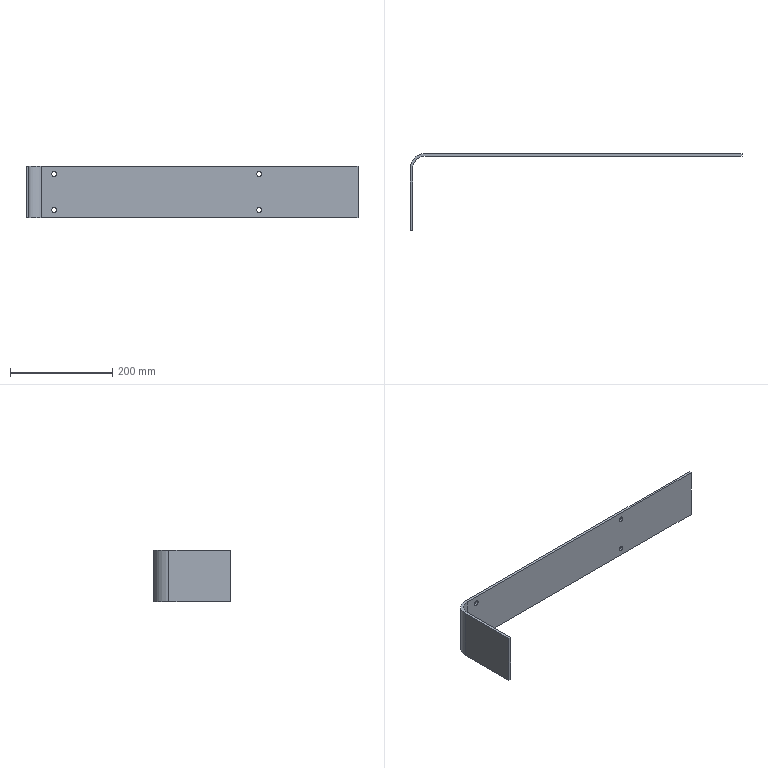Part | SolidWorks | features ExtruThin 1, ICE 1, LPattern 1 | 1 solid | 18 faces | box 648 x 150 x 100 mm | volume 389028 mm3 | cylinder 10 | plane 8 | commonest cylinder face diameters 10 x8 50 x1 60 x1
STEP:
#1=CARTESIAN_POINT('',(455.,150.,10.));
#2=VERTEX_POINT('',#1);
#3=CARTESIAN_POINT('',(455.,150.,20.));
#4=VERTEX_POINT('',#3);
#5=CARTESIAN_POINT('',(455.,150.,15.));
#6=DIRECTION('',(0.,1.,0.));
#7=DIRECTION('',(0.,0.,1.));
#8=AXIS2_PLACEMENT_3D('',#5,#6,#7);
#9=CIRCLE('',#8,5.);
#10=EDGE_CURVE('',#2,#4,#9,.T.);
#11=ORIENTED_EDGE('',*,*,#10,.T.);
#12=CARTESIAN_POINT('',(455.,145.,20.));
#13=VERTEX_POINT('',#12);
#14=CARTESIAN_POINT('',(455.,155.,20.));
#15=DIRECTION('',(0.,-1.,0.));
#16=VECTOR('',#15,1000.);
#17=LINE('',#14,#16);
#18=EDGE_CURVE('',#4,#13,#17,.T.);
#19=ORIENTED_EDGE('',*,*,#18,.T.);
#20=CARTESIAN_POINT('',(455.,145.,10.));
#21=VERTEX_POINT('',#20);
#22=CARTESIAN_POINT('',(455.,145.,15.));
#23=DIRECTION('',(0.,-1.,0.));
#24=DIRECTION('',(0.,0.,-1.));
#25=AXIS2_PLACEMENT_3D('',#22,#23,#24);
#26=CIRCLE('',#25,5.);
#27=EDGE_CURVE('',#13,#21,#26,.T.);
#28=ORIENTED_EDGE('',*,*,#27,.T.);
#29=CARTESIAN_POINT('',(455.,155.,10.));
#30=DIRECTION('',(0.,-1.,0.));
#31=VECTOR('',#30,1000.);
#32=LINE('',#29,#31);
#33=EDGE_CURVE('',#2,#21,#32,.T.);
#34=ORIENTED_EDGE('',*,*,#33,.F.);
#35=EDGE_LOOP('',(#11,#19,#28,#34));
#36=FACE_OUTER_BOUND('',#35,.T.);
#37=CARTESIAN_POINT('',(455.,155.,15.));
#38=DIRECTION('',(0.,-1.,0.));
#39=DIRECTION('',(0.,0.,-1.));
#40=AXIS2_PLACEMENT_3D('',#37,#38,#39);
#41=CYLINDRICAL_SURFACE('',#40,5.);
#42=ADVANCED_FACE('',(#36),#41,.F.);
#43=CARTESIAN_POINT('',(55.,150.,10.));
#44=VERTEX_POINT('',#43);
#45=CARTESIAN_POINT('',(55.,150.,20.));
#46=VERTEX_POINT('',#45);
#47=CARTESIAN_POINT('',(55.,150.,15.));
#48=DIRECTION('',(0.,1.,0.));
#49=DIRECTION('',(0.,0.,1.));
#50=AXIS2_PLACEMENT_3D('',#47,#48,#49);
#51=CIRCLE('',#50,5.);
#52=EDGE_CURVE('',#44,#46,#51,.T.);
#53=ORIENTED_EDGE('',*,*,#52,.T.);
#54=CARTESIAN_POINT('',(55.,145.,20.));
#55=VERTEX_POINT('',#54);
#56=CARTESIAN_POINT('',(55.,155.,20.));
#57=DIRECTION('',(0.,-1.,0.));
#58=VECTOR('',#57,1000.);
#59=LINE('',#56,#58);
#60=EDGE_CURVE('',#46,#55,#59,.T.);
#61=ORIENTED_EDGE('',*,*,#60,.T.);
#62=CARTESIAN_POINT('',(55.,145.,10.));
#63=VERTEX_POINT('',#62);
#64=CARTESIAN_POINT('',(55.,145.,15.));
#65=DIRECTION('',(0.,-1.,0.));
#66=DIRECTION('',(0.,0.,-1.));
#67=AXIS2_PLACEMENT_3D('',#64,#65,#66);
#68=CIRCLE('',#67,5.);
#69=EDGE_CURVE('',#55,#63,#68,.T.);
#70=ORIENTED_EDGE('',*,*,#69,.T.);
#71=CARTESIAN_POINT('',(55.,155.,10.));
#72=DIRECTION('',(0.,-1.,0.));
#73=VECTOR('',#72,1000.);
#74=LINE('',#71,#73);
#75=EDGE_CURVE('',#44,#63,#74,.T.);
#76=ORIENTED_EDGE('',*,*,#75,.F.);
#77=EDGE_LOOP('',(#53,#61,#70,#76));
#78=FACE_OUTER_BOUND('',#77,.T.);
#79=CARTESIAN_POINT('',(55.,155.,15.));
#80=DIRECTION('',(0.,-1.,0.));
#81=DIRECTION('',(0.,0.,-1.));
#82=AXIS2_PLACEMENT_3D('',#79,#80,#81);
#83=CYLINDRICAL_SURFACE('',#82,5.);
#84=ADVANCED_FACE('',(#78),#83,.F.);
#85=CARTESIAN_POINT('',(455.,150.,80.));
#86=VERTEX_POINT('',#85);
#87=CARTESIAN_POINT('',(455.,150.,90.));
#88=VERTEX_POINT('',#87);
#89=CARTESIAN_POINT('',(455.,150.,85.));
#90=DIRECTION('',(0.,1.,0.));
#91=DIRECTION('',(0.,0.,1.));
#92=AXIS2_PLACEMENT_3D('',#89,#90,#91);
#93=CIRCLE('',#92,5.);
#94=EDGE_CURVE('',#86,#88,#93,.T.);
#95=ORIENTED_EDGE('',*,*,#94,.T.);
#96=CARTESIAN_POINT('',(455.,145.,90.));
#97=VERTEX_POINT('',#96);
#98=CARTESIAN_POINT('',(455.,155.,90.));
#99=DIRECTION('',(0.,-1.,0.));
#100=VECTOR('',#99,1000.);
#101=LINE('',#98,#100);
#102=EDGE_CURVE('',#88,#97,#101,.T.);
#103=ORIENTED_EDGE('',*,*,#102,.T.);
#104=CARTESIAN_POINT('',(455.,145.,80.));
#105=VERTEX_POINT('',#104);
#106=CARTESIAN_POINT('',(455.,145.,85.));
#107=DIRECTION('',(0.,-1.,0.));
#108=DIRECTION('',(0.,0.,-1.));
#109=AXIS2_PLACEMENT_3D('',#106,#107,#108);
#110=CIRCLE('',#109,5.);
#111=EDGE_CURVE('',#97,#105,#110,.T.);
#112=ORIENTED_EDGE('',*,*,#111,.T.);
#113=CARTESIAN_POINT('',(455.,155.,80.));
#114=DIRECTION('',(0.,-1.,0.));
#115=VECTOR('',#114,1000.);
#116=LINE('',#113,#115);
#117=EDGE_CURVE('',#86,#105,#116,.T.);
#118=ORIENTED_EDGE('',*,*,#117,.F.);
#119=EDGE_LOOP('',(#95,#103,#112,#118));
#120=FACE_OUTER_BOUND('',#119,.T.);
#121=CARTESIAN_POINT('',(455.,155.,85.));
#122=DIRECTION('',(0.,-1.,0.));
#123=DIRECTION('',(0.,0.,-1.));
#124=AXIS2_PLACEMENT_3D('',#121,#122,#123);
#125=CYLINDRICAL_SURFACE('',#124,5.);
#126=ADVANCED_FACE('',(#120),#125,.F.);
#127=CARTESIAN_POINT('',(55.,150.,80.));
#128=VERTEX_POINT('',#127);
#129=CARTESIAN_POINT('',(55.,150.,90.));
#130=VERTEX_POINT('',#129);
#131=CARTESIAN_POINT('',(55.,150.,85.));
#132=DIRECTION('',(0.,1.,0.));
#133=DIRECTION('',(0.,0.,1.));
#134=AXIS2_PLACEMENT_3D('',#131,#132,#133);
#135=CIRCLE('',#134,5.);
#136=EDGE_CURVE('',#128,#130,#135,.T.);
#137=ORIENTED_EDGE('',*,*,#136,.T.);
#138=CARTESIAN_POINT('',(55.,145.,90.));
#139=VERTEX_POINT('',#138);
#140=CARTESIAN_POINT('',(55.,155.,90.));
#141=DIRECTION('',(0.,-1.,0.));
#142=VECTOR('',#141,1000.);
#143=LINE('',#140,#142);
#144=EDGE_CURVE('',#130,#139,#143,.T.);
#145=ORIENTED_EDGE('',*,*,#144,.T.);
#146=CARTESIAN_POINT('',(55.,145.,80.));
#147=VERTEX_POINT('',#146);
#148=CARTESIAN_POINT('',(55.,145.,85.));
#149=DIRECTION('',(0.,-1.,0.));
#150=DIRECTION('',(0.,0.,-1.));
#151=AXIS2_PLACEMENT_3D('',#148,#149,#150);
#152=CIRCLE('',#151,5.);
#153=EDGE_CURVE('',#139,#147,#152,.T.);
#154=ORIENTED_EDGE('',*,*,#153,.T.);
#155=CARTESIAN_POINT('',(55.,155.,80.));
#156=DIRECTION('',(0.,-1.,0.));
#157=VECTOR('',#156,1000.);
#158=LINE('',#155,#157);
#159=EDGE_CURVE('',#128,#147,#158,.T.);
#160=ORIENTED_EDGE('',*,*,#159,.F.);
#161=EDGE_LOOP('',(#137,#145,#154,#160));
#162=FACE_OUTER_BOUND('',#161,.T.);
#163=CARTESIAN_POINT('',(55.,155.,85.));
#164=DIRECTION('',(0.,-1.,0.));
#165=DIRECTION('',(0.,0.,-1.));
#166=AXIS2_PLACEMENT_3D('',#163,#164,#165);
#167=CYLINDRICAL_SURFACE('',#166,5.);
#168=ADVANCED_FACE('',(#162),#167,.F.);
#169=CARTESIAN_POINT('',(455.,145.,85.));
#170=DIRECTION('',(0.,-1.,0.));
#171=DIRECTION('',(0.,0.,-1.));
#172=AXIS2_PLACEMENT_3D('',#169,#170,#171);
#173=CIRCLE('',#172,5.);
#174=EDGE_CURVE('',#105,#97,#173,.T.);
#175=ORIENTED_EDGE('',*,*,#174,.F.);
#176=ORIENTED_EDGE('',*,*,#111,.F.);
#177=EDGE_LOOP('',(#175,#176));
#178=FACE_BOUND('',#177,.T.);
#179=CARTESIAN_POINT('',(55.,145.,85.));
#180=DIRECTION('',(0.,-1.,0.));
#181=DIRECTION('',(0.,0.,-1.));
#182=AXIS2_PLACEMENT_3D('',#179,#180,#181);
#183=CIRCLE('',#182,5.);
#184=EDGE_CURVE('',#147,#139,#183,.T.);
#185=ORIENTED_EDGE('',*,*,#184,.F.);
#186=ORIENTED_EDGE('',*,*,#153,.F.);
#187=EDGE_LOOP('',(#185,#186));
#188=FACE_BOUND('',#187,.T.);
#189=CARTESIAN_POINT('',(30.,145.,0.));
#190=VERTEX_POINT('',#189);
#191=CARTESIAN_POINT('',(648.,145.,0.));
#192=VERTEX_POINT('',#191);
#193=CARTESIAN_POINT('',(30.,145.,0.));
#194=DIRECTION('',(1.,0.,0.));
#195=VECTOR('',#194,1000.);
#196=LINE('',#193,#195);
#197=EDGE_CURVE('',#190,#192,#196,.T.);
#198=ORIENTED_EDGE('',*,*,#197,.T.);
#199=CARTESIAN_POINT('',(648.,145.,100.));
#200=VERTEX_POINT('',#199);
#201=CARTESIAN_POINT('',(648.,145.,100.));
#202=DIRECTION('',(0.,0.,-1.));
#203=VECTOR('',#202,1000.);
#204=LINE('',#201,#203);
#205=EDGE_CURVE('',#200,#192,#204,.T.);
#206=ORIENTED_EDGE('',*,*,#205,.F.);
#207=CARTESIAN_POINT('',(30.,145.,100.));
#208=VERTEX_POINT('',#207);
#209=CARTESIAN_POINT('',(30.,145.,100.));
#210=DIRECTION('',(1.,0.,0.));
#211=VECTOR('',#210,1000.);
#212=LINE('',#209,#211);
#213=EDGE_CURVE('',#208,#200,#212,.T.);
#214=ORIENTED_EDGE('',*,*,#213,.F.);
#215=CARTESIAN_POINT('',(30.,145.,100.));
#216=DIRECTION('',(0.,0.,-1.));
#217=VECTOR('',#216,1000.);
#218=LINE('',#215,#217);
#219=EDGE_CURVE('',#208,#190,#218,.T.);
#220=ORIENTED_EDGE('',*,*,#219,.T.);
#221=EDGE_LOOP('',(#198,#206,#214,#220));
#222=FACE_OUTER_BOUND('',#221,.T.);
#223=CARTESIAN_POINT('',(55.,145.,15.));
#224=DIRECTION('',(0.,-1.,0.));
#225=DIRECTION('',(0.,0.,-1.));
#226=AXIS2_PLACEMENT_3D('',#223,#224,#225);
#227=CIRCLE('',#226,5.);
#228=EDGE_CURVE('',#63,#55,#227,.T.);
#229=ORIENTED_EDGE('',*,*,#228,.F.);
#230=ORIENTED_EDGE('',*,*,#69,.F.);
#231=EDGE_LOOP('',(#229,#230));
#232=FACE_BOUND('',#231,.T.);
#233=CARTESIAN_POINT('',(455.,145.,15.));
#234=DIRECTION('',(0.,-1.,0.));
#235=DIRECTION('',(0.,0.,-1.));
#236=AXIS2_PLACEMENT_3D('',#233,#234,#235);
#237=CIRCLE('',#236,5.);
#238=EDGE_CURVE('',#21,#13,#237,.T.);
#239=ORIENTED_EDGE('',*,*,#238,.F.);
#240=ORIENTED_EDGE('',*,*,#27,.F.);
#241=EDGE_LOOP('',(#239,#240));
#242=FACE_BOUND('',#241,.T.);
#243=CARTESIAN_POINT('',(30.,145.,100.));
#244=DIRECTION('',(0.,1.,0.));
#245=DIRECTION('',(0.,0.,1.));
#246=AXIS2_PLACEMENT_3D('',#243,#244,#245);
#247=PLANE('',#246);
#248=ADVANCED_FACE('',(#178,#188,#222,#232,#242),#247,.F.);
#249=CARTESIAN_POINT('',(648.,150.,0.));
#250=VERTEX_POINT('',#249);
#251=CARTESIAN_POINT('',(648.,150.,0.));
#252=DIRECTION('',(0.,-1.,0.));
#253=VECTOR('',#252,1000.);
#254=LINE('',#251,#253);
#255=EDGE_CURVE('',#250,#192,#254,.T.);
#256=ORIENTED_EDGE('',*,*,#255,.F.);
#257=CARTESIAN_POINT('',(648.,150.,100.));
#258=VERTEX_POINT('',#257);
#259=CARTESIAN_POINT('',(648.,150.,100.));
#260=DIRECTION('',(0.,0.,-1.));
#261=VECTOR('',#260,1000.);
#262=LINE('',#259,#261);
#263=EDGE_CURVE('',#258,#250,#262,.T.);
#264=ORIENTED_EDGE('',*,*,#263,.F.);
#265=CARTESIAN_POINT('',(648.,150.,100.));
#266=DIRECTION('',(0.,-1.,0.));
#267=VECTOR('',#266,1000.);
#268=LINE('',#265,#267);
#269=EDGE_CURVE('',#258,#200,#268,.T.);
#270=ORIENTED_EDGE('',*,*,#269,.T.);
#271=ORIENTED_EDGE('',*,*,#205,.T.);
#272=EDGE_LOOP('',(#256,#264,#270,#271));
#273=FACE_OUTER_BOUND('',#272,.T.);
#274=CARTESIAN_POINT('',(648.,150.,100.));
#275=DIRECTION('',(1.,0.,0.));
#276=DIRECTION('',(0.,0.,-1.));
#277=AXIS2_PLACEMENT_3D('',#274,#275,#276);
#278=PLANE('',#277);
#279=ADVANCED_FACE('',(#273),#278,.T.);
#280=ORIENTED_EDGE('',*,*,#94,.F.);
#281=CARTESIAN_POINT('',(455.,150.,85.));
#282=DIRECTION('',(0.,1.,0.));
#283=DIRECTION('',(0.,0.,1.));
#284=AXIS2_PLACEMENT_3D('',#281,#282,#283);
#285=CIRCLE('',#284,5.);
#286=EDGE_CURVE('',#88,#86,#285,.T.);
#287=ORIENTED_EDGE('',*,*,#286,.F.);
#288=EDGE_LOOP('',(#280,#287));
#289=FACE_BOUND('',#288,.T.);
#290=ORIENTED_EDGE('',*,*,#136,.F.);
#291=CARTESIAN_POINT('',(55.,150.,85.));
#292=DIRECTION('',(0.,1.,0.));
#293=DIRECTION('',(0.,0.,1.));
#294=AXIS2_PLACEMENT_3D('',#291,#292,#293);
#295=CIRCLE('',#294,5.);
#296=EDGE_CURVE('',#130,#128,#295,.T.);
#297=ORIENTED_EDGE('',*,*,#296,.F.);
#298=EDGE_LOOP('',(#290,#297));
#299=FACE_BOUND('',#298,.T.);
#300=CARTESIAN_POINT('',(30.,150.,0.));
#301=VERTEX_POINT('',#300);
#302=CARTESIAN_POINT('',(30.,150.,0.));
#303=DIRECTION('',(1.,0.,0.));
#304=VECTOR('',#303,1000.);
#305=LINE('',#302,#304);
#306=EDGE_CURVE('',#301,#250,#305,.T.);
#307=ORIENTED_EDGE('',*,*,#306,.F.);
#308=CARTESIAN_POINT('',(30.,150.,100.));
#309=VERTEX_POINT('',#308);
#310=CARTESIAN_POINT('',(30.,150.,100.));
#311=DIRECTION('',(0.,0.,-1.));
#312=VECTOR('',#311,1000.);
#313=LINE('',#310,#312);
#314=EDGE_CURVE('',#309,#301,#313,.T.);
#315=ORIENTED_EDGE('',*,*,#314,.F.);
#316=CARTESIAN_POINT('',(30.,150.,100.));
#317=DIRECTION('',(1.,0.,0.));
#318=VECTOR('',#317,1000.);
#319=LINE('',#316,#318);
#320=EDGE_CURVE('',#309,#258,#319,.T.);
#321=ORIENTED_EDGE('',*,*,#320,.T.);
#322=ORIENTED_EDGE('',*,*,#263,.T.);
#323=EDGE_LOOP('',(#307,#315,#321,#322));
#324=FACE_OUTER_BOUND('',#323,.T.);
#325=ORIENTED_EDGE('',*,*,#52,.F.);
#326=CARTESIAN_POINT('',(55.,150.,15.));
#327=DIRECTION('',(0.,1.,0.));
#328=DIRECTION('',(0.,0.,1.));
#329=AXIS2_PLACEMENT_3D('',#326,#327,#328);
#330=CIRCLE('',#329,5.);
#331=EDGE_CURVE('',#46,#44,#330,.T.);
#332=ORIENTED_EDGE('',*,*,#331,.F.);
#333=EDGE_LOOP('',(#325,#332));
#334=FACE_BOUND('',#333,.T.);
#335=ORIENTED_EDGE('',*,*,#10,.F.);
#336=CARTESIAN_POINT('',(455.,150.,15.));
#337=DIRECTION('',(0.,1.,0.));
#338=DIRECTION('',(0.,0.,1.));
#339=AXIS2_PLACEMENT_3D('',#336,#337,#338);
#340=CIRCLE('',#339,5.);
#341=EDGE_CURVE('',#4,#2,#340,.T.);
#342=ORIENTED_EDGE('',*,*,#341,.F.);
#343=EDGE_LOOP('',(#335,#342));
#344=FACE_BOUND('',#343,.T.);
#345=CARTESIAN_POINT('',(30.,150.,100.));
#346=DIRECTION('',(0.,1.,0.));
#347=DIRECTION('',(0.,0.,1.));
#348=AXIS2_PLACEMENT_3D('',#345,#346,#347);
#349=PLANE('',#348);
#350=ADVANCED_FACE('',(#289,#299,#324,#334,#344),#349,.T.);
#351=CARTESIAN_POINT('',(0.,120.,0.));
#352=VERTEX_POINT('',#351);
#353=CARTESIAN_POINT('',(30.,120.,0.));
#354=DIRECTION('',(0.,0.,-1.));
#355=DIRECTION('',(1.,0.,0.));
#356=AXIS2_PLACEMENT_3D('',#353,#354,#355);
#357=CIRCLE('',#356,30.);
#358=EDGE_CURVE('',#352,#301,#357,.T.);
#359=ORIENTED_EDGE('',*,*,#358,.F.);
#360=CARTESIAN_POINT('',(0.,120.,100.));
#361=VERTEX_POINT('',#360);
#362=CARTESIAN_POINT('',(0.,120.,100.));
#363=DIRECTION('',(0.,0.,-1.));
#364=VECTOR('',#363,1000.);
#365=LINE('',#362,#364);
#366=EDGE_CURVE('',#361,#352,#365,.T.);
#367=ORIENTED_EDGE('',*,*,#366,.F.);
#368=CARTESIAN_POINT('',(30.,120.,100.));
#369=DIRECTION('',(0.,0.,-1.));
#370=DIRECTION('',(1.,0.,0.));
#371=AXIS2_PLACEMENT_3D('',#368,#369,#370);
#372=CIRCLE('',#371,30.);
#373=EDGE_CURVE('',#361,#309,#372,.T.);
#374=ORIENTED_EDGE('',*,*,#373,.T.);
#375=ORIENTED_EDGE('',*,*,#314,.T.);
#376=EDGE_LOOP('',(#359,#367,#374,#375));
#377=FACE_OUTER_BOUND('',#376,.T.);
#378=CARTESIAN_POINT('',(30.,120.,100.));
#379=DIRECTION('',(0.,0.,-1.));
#380=DIRECTION('',(-1.,0.,0.));
#381=AXIS2_PLACEMENT_3D('',#378,#379,#380);
#382=CYLINDRICAL_SURFACE('',#381,30.);
#383=ADVANCED_FACE('',(#377),#382,.T.);
#384=CARTESIAN_POINT('',(0.,0.,0.));
#385=VERTEX_POINT('',#384);
#386=CARTESIAN_POINT('',(0.,0.,0.));
#387=DIRECTION('',(0.,1.,0.));
#388=VECTOR('',#387,1000.);
#389=LINE('',#386,#388);
#390=EDGE_CURVE('',#385,#352,#389,.T.);
#391=ORIENTED_EDGE('',*,*,#390,.F.);
#392=CARTESIAN_POINT('',(0.,0.,100.));
#393=VERTEX_POINT('',#392);
#394=CARTESIAN_POINT('',(0.,0.,100.));
#395=DIRECTION('',(0.,0.,-1.));
#396=VECTOR('',#395,1000.);
#397=LINE('',#394,#396);
#398=EDGE_CURVE('',#393,#385,#397,.T.);
#399=ORIENTED_EDGE('',*,*,#398,.F.);
#400=CARTESIAN_POINT('',(0.,0.,100.));
#401=DIRECTION('',(0.,1.,0.));
#402=VECTOR('',#401,1000.);
#403=LINE('',#400,#402);
#404=EDGE_CURVE('',#393,#361,#403,.T.);
#405=ORIENTED_EDGE('',*,*,#404,.T.);
#406=ORIENTED_EDGE('',*,*,#366,.T.);
#407=EDGE_LOOP('',(#391,#399,#405,#406));
#408=FACE_OUTER_BOUND('',#407,.T.);
#409=CARTESIAN_POINT('',(0.,0.,100.));
#410=DIRECTION('',(-1.,0.,0.));
#411=DIRECTION('',(0.,0.,1.));
#412=AXIS2_PLACEMENT_3D('',#409,#410,#411);
#413=PLANE('',#412);
#414=ADVANCED_FACE('',(#408),#413,.T.);
#415=CARTESIAN_POINT('',(5.,0.,0.));
#416=VERTEX_POINT('',#415);
#417=CARTESIAN_POINT('',(5.,0.,0.));
#418=DIRECTION('',(-1.,0.,0.));
#419=VECTOR('',#418,1000.);
#420=LINE('',#417,#419);
#421=EDGE_CURVE('',#416,#385,#420,.T.);
#422=ORIENTED_EDGE('',*,*,#421,.F.);
#423=CARTESIAN_POINT('',(5.,0.,100.));
#424=VERTEX_POINT('',#423);
#425=CARTESIAN_POINT('',(5.,0.,100.));
#426=DIRECTION('',(0.,0.,-1.));
#427=VECTOR('',#426,1000.);
#428=LINE('',#425,#427);
#429=EDGE_CURVE('',#424,#416,#428,.T.);
#430=ORIENTED_EDGE('',*,*,#429,.F.);
#431=CARTESIAN_POINT('',(5.,0.,100.));
#432=DIRECTION('',(-1.,0.,0.));
#433=VECTOR('',#432,1000.);
#434=LINE('',#431,#433);
#435=EDGE_CURVE('',#424,#393,#434,.T.);
#436=ORIENTED_EDGE('',*,*,#435,.T.);
#437=ORIENTED_EDGE('',*,*,#398,.T.);
#438=EDGE_LOOP('',(#422,#430,#436,#437));
#439=FACE_OUTER_BOUND('',#438,.T.);
#440=CARTESIAN_POINT('',(5.,0.,100.));
#441=DIRECTION('',(0.,-1.,0.));
#442=DIRECTION('',(0.,0.,-1.));
#443=AXIS2_PLACEMENT_3D('',#440,#441,#442);
#444=PLANE('',#443);
#445=ADVANCED_FACE('',(#439),#444,.T.);
#446=CARTESIAN_POINT('',(5.,120.,0.));
#447=VERTEX_POINT('',#446);
#448=CARTESIAN_POINT('',(5.,0.,0.));
#449=DIRECTION('',(0.,1.,0.));
#450=VECTOR('',#449,1000.);
#451=LINE('',#448,#450);
#452=EDGE_CURVE('',#416,#447,#451,.T.);
#453=ORIENTED_EDGE('',*,*,#452,.T.);
#454=CARTESIAN_POINT('',(5.,120.,100.));
#455=VERTEX_POINT('',#454);
#456=CARTESIAN_POINT('',(5.,120.,100.));
#457=DIRECTION('',(0.,0.,-1.));
#458=VECTOR('',#457,1000.);
#459=LINE('',#456,#458);
#460=EDGE_CURVE('',#455,#447,#459,.T.);
#461=ORIENTED_EDGE('',*,*,#460,.F.);
#462=CARTESIAN_POINT('',(5.,0.,100.));
#463=DIRECTION('',(0.,1.,0.));
#464=VECTOR('',#463,1000.);
#465=LINE('',#462,#464);
#466=EDGE_CURVE('',#424,#455,#465,.T.);
#467=ORIENTED_EDGE('',*,*,#466,.F.);
#468=ORIENTED_EDGE('',*,*,#429,.T.);
#469=EDGE_LOOP('',(#453,#461,#467,#468));
#470=FACE_OUTER_BOUND('',#469,.T.);
#471=CARTESIAN_POINT('',(5.,0.,100.));
#472=DIRECTION('',(-1.,0.,0.));
#473=DIRECTION('',(0.,0.,1.));
#474=AXIS2_PLACEMENT_3D('',#471,#472,#473);
#475=PLANE('',#474);
#476=ADVANCED_FACE('',(#470),#475,.F.);
#477=CARTESIAN_POINT('',(30.,120.,0.));
#478=DIRECTION('',(0.,0.,-1.));
#479=DIRECTION('',(1.,0.,0.));
#480=AXIS2_PLACEMENT_3D('',#477,#478,#479);
#481=CIRCLE('',#480,25.);
#482=EDGE_CURVE('',#447,#190,#481,.T.);
#483=ORIENTED_EDGE('',*,*,#482,.T.);
#484=ORIENTED_EDGE('',*,*,#219,.F.);
#485=CARTESIAN_POINT('',(30.,120.,100.));
#486=DIRECTION('',(0.,0.,-1.));
#487=DIRECTION('',(1.,0.,0.));
#488=AXIS2_PLACEMENT_3D('',#485,#486,#487);
#489=CIRCLE('',#488,25.);
#490=EDGE_CURVE('',#455,#208,#489,.T.);
#491=ORIENTED_EDGE('',*,*,#490,.F.);
#492=ORIENTED_EDGE('',*,*,#460,.T.);
#493=EDGE_LOOP('',(#483,#484,#491,#492));
#494=FACE_OUTER_BOUND('',#493,.T.);
#495=CARTESIAN_POINT('',(30.,120.,100.));
#496=DIRECTION('',(0.,0.,-1.));
#497=DIRECTION('',(-1.,0.,0.));
#498=AXIS2_PLACEMENT_3D('',#495,#496,#497);
#499=CYLINDRICAL_SURFACE('',#498,25.);
#500=ADVANCED_FACE('',(#494),#499,.F.);
#501=ORIENTED_EDGE('',*,*,#213,.T.);
#502=ORIENTED_EDGE('',*,*,#269,.F.);
#503=ORIENTED_EDGE('',*,*,#320,.F.);
#504=ORIENTED_EDGE('',*,*,#373,.F.);
#505=ORIENTED_EDGE('',*,*,#404,.F.);
#506=ORIENTED_EDGE('',*,*,#435,.F.);
#507=ORIENTED_EDGE('',*,*,#466,.T.);
#508=ORIENTED_EDGE('',*,*,#490,.T.);
#509=EDGE_LOOP('',(#501,#502,#503,#504,#505,#506,#507,#508));
#510=FACE_OUTER_BOUND('',#509,.T.);
#511=CARTESIAN_POINT('',(30.,120.,100.));
#512=DIRECTION('',(0.,0.,-1.));
#513=DIRECTION('',(-1.,0.,0.));
#514=AXIS2_PLACEMENT_3D('',#511,#512,#513);
#515=PLANE('',#514);
#516=ADVANCED_FACE('',(#510),#515,.F.);
#517=ORIENTED_EDGE('',*,*,#197,.F.);
#518=ORIENTED_EDGE('',*,*,#482,.F.);
#519=ORIENTED_EDGE('',*,*,#452,.F.);
#520=ORIENTED_EDGE('',*,*,#421,.T.);
#521=ORIENTED_EDGE('',*,*,#390,.T.);
#522=ORIENTED_EDGE('',*,*,#358,.T.);
#523=ORIENTED_EDGE('',*,*,#306,.T.);
#524=ORIENTED_EDGE('',*,*,#255,.T.);
#525=EDGE_LOOP('',(#517,#518,#519,#520,#521,#522,#523,#524));
#526=FACE_OUTER_BOUND('',#525,.T.);
#527=CARTESIAN_POINT('',(30.,120.,0.));
#528=DIRECTION('',(0.,0.,-1.));
#529=DIRECTION('',(-1.,0.,0.));
#530=AXIS2_PLACEMENT_3D('',#527,#528,#529);
#531=PLANE('',#530);
#532=ADVANCED_FACE('',(#526),#531,.T.);
#533=ORIENTED_EDGE('',*,*,#144,.F.);
#534=ORIENTED_EDGE('',*,*,#296,.T.);
#535=ORIENTED_EDGE('',*,*,#159,.T.);
#536=ORIENTED_EDGE('',*,*,#184,.T.);
#537=EDGE_LOOP('',(#533,#534,#535,#536));
#538=FACE_OUTER_BOUND('',#537,.T.);
#539=CARTESIAN_POINT('',(55.,155.,85.));
#540=DIRECTION('',(0.,-1.,0.));
#541=DIRECTION('',(0.,0.,-1.));
#542=AXIS2_PLACEMENT_3D('',#539,#540,#541);
#543=CYLINDRICAL_SURFACE('',#542,5.);
#544=ADVANCED_FACE('',(#538),#543,.F.);
#545=ORIENTED_EDGE('',*,*,#102,.F.);
#546=ORIENTED_EDGE('',*,*,#286,.T.);
#547=ORIENTED_EDGE('',*,*,#117,.T.);
#548=ORIENTED_EDGE('',*,*,#174,.T.);
#549=EDGE_LOOP('',(#545,#546,#547,#548));
#550=FACE_OUTER_BOUND('',#549,.T.);
#551=CARTESIAN_POINT('',(455.,155.,85.));
#552=DIRECTION('',(0.,-1.,0.));
#553=DIRECTION('',(0.,0.,-1.));
#554=AXIS2_PLACEMENT_3D('',#551,#552,#553);
#555=CYLINDRICAL_SURFACE('',#554,5.);
#556=ADVANCED_FACE('',(#550),#555,.F.);
#557=ORIENTED_EDGE('',*,*,#60,.F.);
#558=ORIENTED_EDGE('',*,*,#331,.T.);
#559=ORIENTED_EDGE('',*,*,#75,.T.);
#560=ORIENTED_EDGE('',*,*,#228,.T.);
#561=EDGE_LOOP('',(#557,#558,#559,#560));
#562=FACE_OUTER_BOUND('',#561,.T.);
#563=CARTESIAN_POINT('',(55.,155.,15.));
#564=DIRECTION('',(0.,-1.,0.));
#565=DIRECTION('',(0.,0.,-1.));
#566=AXIS2_PLACEMENT_3D('',#563,#564,#565);
#567=CYLINDRICAL_SURFACE('',#566,5.);
#568=ADVANCED_FACE('',(#562),#567,.F.);
#569=ORIENTED_EDGE('',*,*,#18,.F.);
#570=ORIENTED_EDGE('',*,*,#341,.T.);
#571=ORIENTED_EDGE('',*,*,#33,.T.);
#572=ORIENTED_EDGE('',*,*,#238,.T.);
#573=EDGE_LOOP('',(#569,#570,#571,#572));
#574=FACE_OUTER_BOUND('',#573,.T.);
#575=CARTESIAN_POINT('',(455.,155.,15.));
#576=DIRECTION('',(0.,-1.,0.));
#577=DIRECTION('',(0.,0.,-1.));
#578=AXIS2_PLACEMENT_3D('',#575,#576,#577);
#579=CYLINDRICAL_SURFACE('',#578,5.);
#580=ADVANCED_FACE('',(#574),#579,.F.);
#581=CLOSED_SHELL('',(#42,#84,#126,#168,#248,#279,#350,#383,#414,#445,#476,#500,#516,#532,#544,#556,#568,#580));
#582=MANIFOLD_SOLID_BREP('',#581);
#583=CARTESIAN_POINT('',(0.,0.,0.));
#584=DIRECTION('',(0.,0.,1.));
#585=DIRECTION('',(1.,0.,0.));
#586=AXIS2_PLACEMENT_3D('',#583,#584,#585);
#587=(LENGTH_UNIT()NAMED_UNIT(*)SI_UNIT(.MILLI.,.METRE.));
#588=UNCERTAINTY_MEASURE_WITH_UNIT(LENGTH_MEASURE(0.00001),#587,'','');
#589=(NAMED_UNIT(*)PLANE_ANGLE_UNIT()SI_UNIT($,.RADIAN.));
#590=(NAMED_UNIT(*)SI_UNIT($,.STERADIAN.)SOLID_ANGLE_UNIT());
#591=(GEOMETRIC_REPRESENTATION_CONTEXT(3)GLOBAL_UNCERTAINTY_ASSIGNED_CONTEXT((#588))GLOBAL_UNIT_ASSIGNED_CONTEXT((#587,#589,#590))REPRESENTATION_CONTEXT('',''));
#592=ADVANCED_BREP_SHAPE_REPRESENTATION('',(#582,#586),#591);